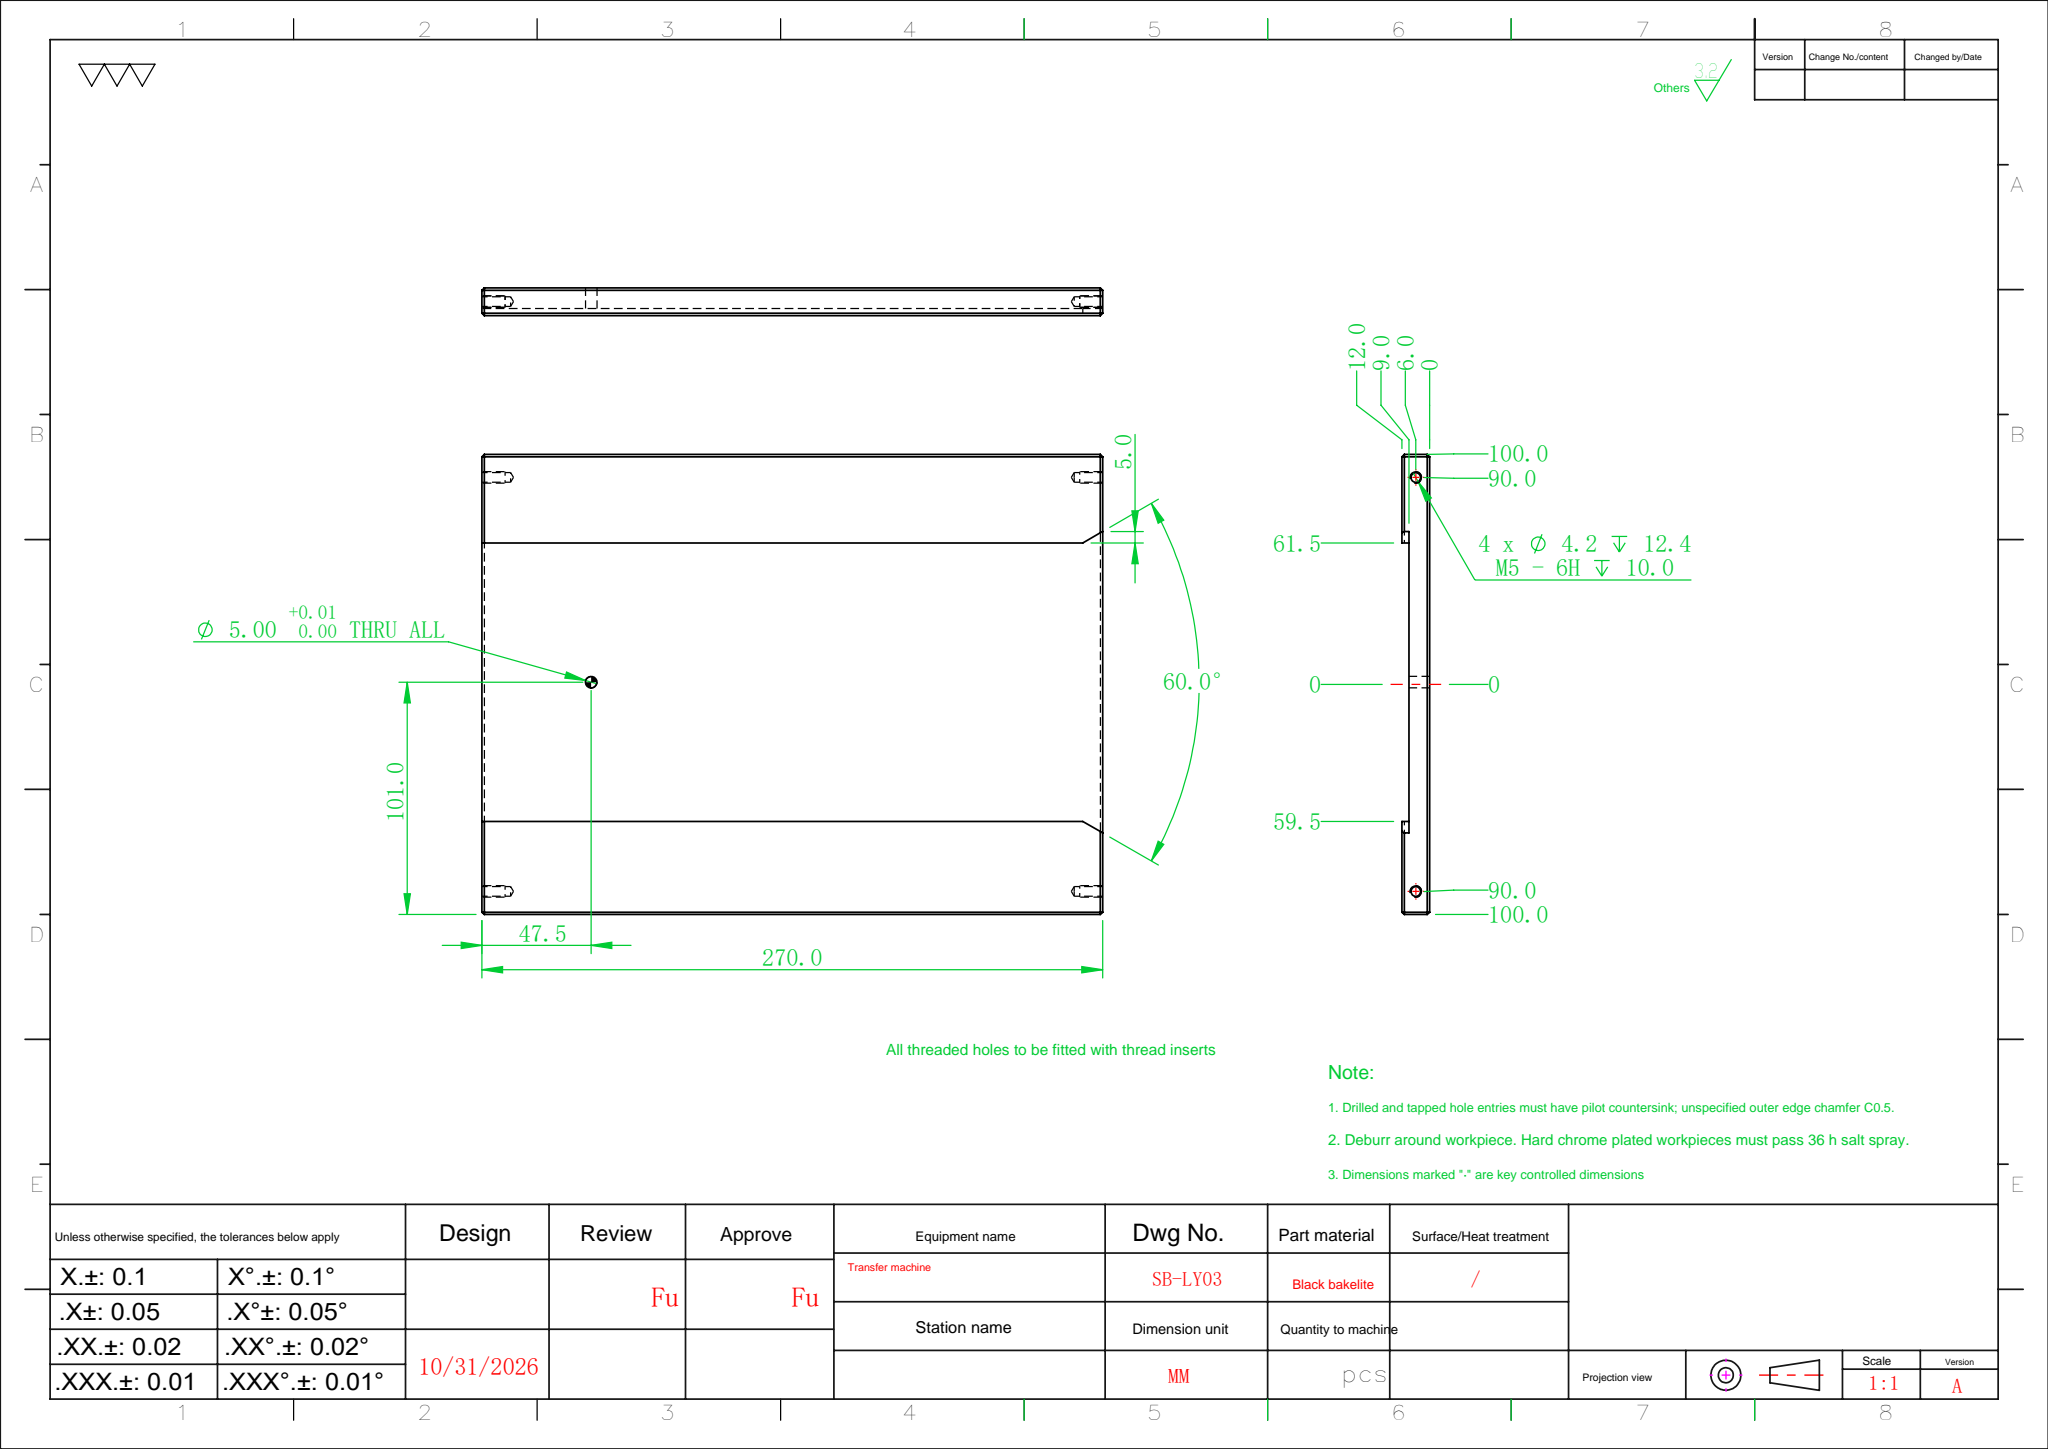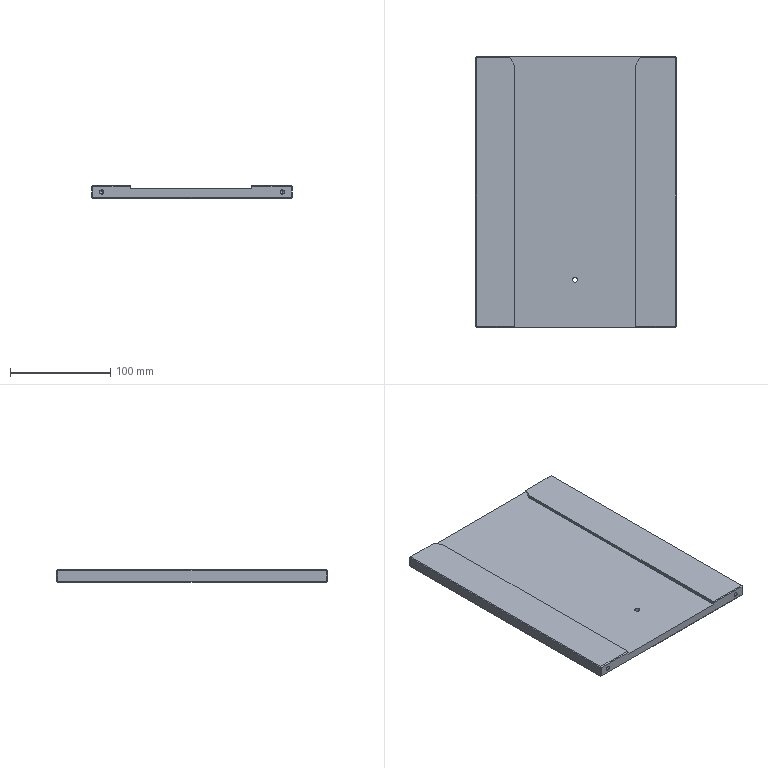Part | SolidWorks | features Chamfer 2, HoleWzd 2, Cut 1, Extrusion 1, MirrorPattern 1 | 1 solid | 52 faces | box 200 x 270 x 12 mm | volume 548140 mm3 | plane 34 | cylinder 10 | cone 8 | commonest cylinder face diameters 4.2 x8 5 x2